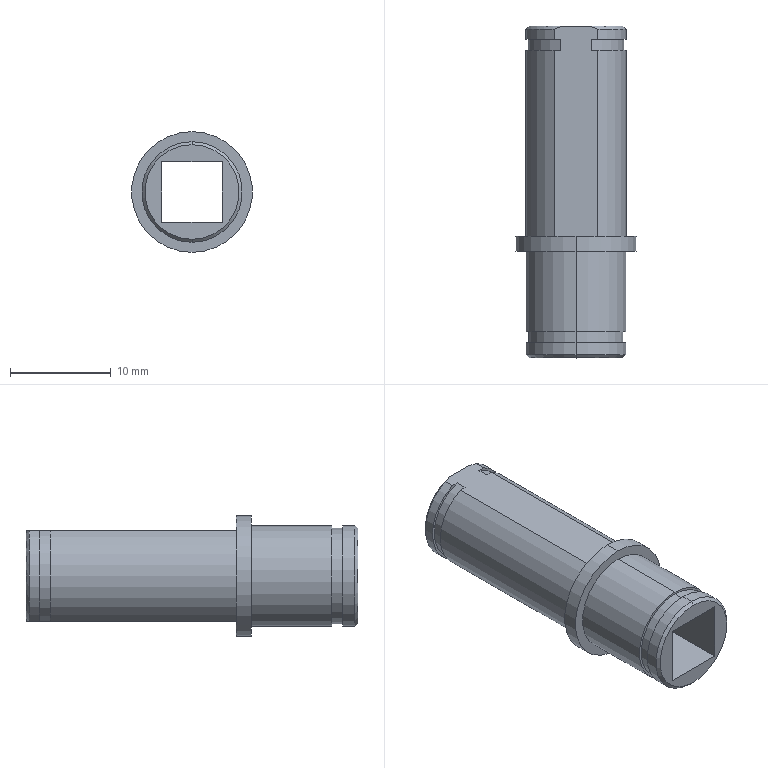Part | NX | features BREP 1 | 1 solid | 34 faces | box 12 x 33 x 12 mm | volume 1377 mm3 | plane 16 | cylinder 14 | cone 4 | commonest cylinder face diameters 10 x8 9.5 x4 12 x2
STEP:
#1=CARTESIAN_POINT('',(0.,0.3,-5.));
#2=VERTEX_POINT('',#1);
#3=CARTESIAN_POINT('',(0.,0.,-4.7));
#4=VERTEX_POINT('',#3);
#5=CARTESIAN_POINT('',(0.,0.,-4.7));
#6=DIRECTION('',(0.,0.7071,-0.7071));
#7=VECTOR('',#6,1000.);
#8=LINE('',#5,#7);
#9=EDGE_CURVE('',#2,#4,#8,.F.);
#10=ORIENTED_EDGE('',*,*,#9,.T.);
#11=CARTESIAN_POINT('',(0.,0.,4.7));
#12=VERTEX_POINT('',#11);
#13=CARTESIAN_POINT('',(0.,0.,0.));
#14=DIRECTION('',(0.,-1.,0.));
#15=DIRECTION('',(0.,0.,1.));
#16=AXIS2_PLACEMENT_3D('',#13,#14,#15);
#17=CIRCLE('',#16,4.7);
#18=EDGE_CURVE('',#12,#4,#17,.T.);
#19=ORIENTED_EDGE('',*,*,#18,.F.);
#20=CARTESIAN_POINT('',(0.,0.3,5.));
#21=VERTEX_POINT('',#20);
#22=CARTESIAN_POINT('',(0.,0.,4.7));
#23=DIRECTION('',(0.,0.7071,0.7071));
#24=VECTOR('',#23,1000.);
#25=LINE('',#22,#24);
#26=EDGE_CURVE('',#21,#12,#25,.F.);
#27=ORIENTED_EDGE('',*,*,#26,.F.);
#28=CARTESIAN_POINT('',(0.,0.3,0.));
#29=DIRECTION('',(0.,1.,0.));
#30=DIRECTION('',(0.,0.,1.));
#31=AXIS2_PLACEMENT_3D('',#28,#29,#30);
#32=CIRCLE('',#31,5.);
#33=EDGE_CURVE('',#2,#21,#32,.T.);
#34=ORIENTED_EDGE('',*,*,#33,.F.);
#35=EDGE_LOOP('',(#10,#19,#27,#34));
#36=FACE_BOUND('',#35,.T.);
#37=CARTESIAN_POINT('',(0.,0.,0.));
#38=DIRECTION('',(0.,1.,0.));
#39=DIRECTION('',(0.,0.,1.));
#40=AXIS2_PLACEMENT_3D('',#37,#38,#39);
#41=CONICAL_SURFACE('',#40,4.7,0.7854);
#42=ADVANCED_FACE('',(#36),#41,.T.);
#43=CARTESIAN_POINT('',(-1.356,33.,4.5));
#44=VERTEX_POINT('',#43);
#45=CARTESIAN_POINT('',(-2.179,32.7,4.5));
#46=VERTEX_POINT('',#45);
#47=CARTESIAN_POINT('',(-1.356,33.,4.5));
#48=CARTESIAN_POINT('',(-1.622,32.923,4.5));
#49=CARTESIAN_POINT('',(-1.897,32.823,4.5));
#50=CARTESIAN_POINT('',(-2.179,32.7,4.5));
#51=B_SPLINE_CURVE_WITH_KNOTS('',3,(#47,#48,#49,#50),.UNSPECIFIED.,.F.,.F.,(4,4),(0.,1.),.UNSPECIFIED.);
#52=EDGE_CURVE('',#44,#46,#51,.T.);
#53=ORIENTED_EDGE('',*,*,#52,.F.);
#54=CARTESIAN_POINT('',(-1.356,33.,-4.5));
#55=VERTEX_POINT('',#54);
#56=CARTESIAN_POINT('',(0.,33.,0.));
#57=DIRECTION('',(0.,1.,0.));
#58=DIRECTION('',(0.,0.,-1.));
#59=AXIS2_PLACEMENT_3D('',#56,#57,#58);
#60=CIRCLE('',#59,4.7);
#61=EDGE_CURVE('',#55,#44,#60,.T.);
#62=ORIENTED_EDGE('',*,*,#61,.F.);
#63=CARTESIAN_POINT('',(-2.179,32.7,-4.5));
#64=VERTEX_POINT('',#63);
#65=CARTESIAN_POINT('',(-2.179,32.7,-4.5));
#66=CARTESIAN_POINT('',(-1.897,32.823,-4.5));
#67=CARTESIAN_POINT('',(-1.622,32.923,-4.5));
#68=CARTESIAN_POINT('',(-1.356,33.,-4.5));
#69=B_SPLINE_CURVE_WITH_KNOTS('',3,(#65,#66,#67,#68),.UNSPECIFIED.,.F.,.F.,(4,4),(0.,1.),.UNSPECIFIED.);
#70=EDGE_CURVE('',#64,#55,#69,.T.);
#71=ORIENTED_EDGE('',*,*,#70,.F.);
#72=CARTESIAN_POINT('',(0.,32.7,0.));
#73=DIRECTION('',(0.,-1.,0.));
#74=DIRECTION('',(0.,0.,-1.));
#75=AXIS2_PLACEMENT_3D('',#72,#73,#74);
#76=CIRCLE('',#75,5.);
#77=EDGE_CURVE('',#46,#64,#76,.T.);
#78=ORIENTED_EDGE('',*,*,#77,.F.);
#79=EDGE_LOOP('',(#53,#62,#71,#78));
#80=FACE_BOUND('',#79,.T.);
#81=CARTESIAN_POINT('',(0.,32.7,0.));
#82=DIRECTION('',(0.,-1.,0.));
#83=DIRECTION('',(0.,0.,-1.));
#84=AXIS2_PLACEMENT_3D('',#81,#82,#83);
#85=CONICAL_SURFACE('',#84,5.,0.7854);
#86=ADVANCED_FACE('',(#80),#85,.T.);
#87=CARTESIAN_POINT('',(1.356,33.,-4.5));
#88=VERTEX_POINT('',#87);
#89=CARTESIAN_POINT('',(2.179,32.7,-4.5));
#90=VERTEX_POINT('',#89);
#91=CARTESIAN_POINT('',(1.356,33.,-4.5));
#92=CARTESIAN_POINT('',(1.622,32.923,-4.5));
#93=CARTESIAN_POINT('',(1.897,32.823,-4.5));
#94=CARTESIAN_POINT('',(2.179,32.7,-4.5));
#95=B_SPLINE_CURVE_WITH_KNOTS('',3,(#91,#92,#93,#94),.UNSPECIFIED.,.F.,.F.,(4,4),(0.,1.),.UNSPECIFIED.);
#96=EDGE_CURVE('',#88,#90,#95,.T.);
#97=ORIENTED_EDGE('',*,*,#96,.F.);
#98=CARTESIAN_POINT('',(1.356,33.,4.5));
#99=VERTEX_POINT('',#98);
#100=CARTESIAN_POINT('',(0.,33.,0.));
#101=DIRECTION('',(0.,1.,0.));
#102=DIRECTION('',(0.,0.,-1.));
#103=AXIS2_PLACEMENT_3D('',#100,#101,#102);
#104=CIRCLE('',#103,4.7);
#105=EDGE_CURVE('',#99,#88,#104,.T.);
#106=ORIENTED_EDGE('',*,*,#105,.F.);
#107=CARTESIAN_POINT('',(2.179,32.7,4.5));
#108=VERTEX_POINT('',#107);
#109=CARTESIAN_POINT('',(2.179,32.7,4.5));
#110=CARTESIAN_POINT('',(1.897,32.823,4.5));
#111=CARTESIAN_POINT('',(1.622,32.923,4.5));
#112=CARTESIAN_POINT('',(1.356,33.,4.5));
#113=B_SPLINE_CURVE_WITH_KNOTS('',3,(#109,#110,#111,#112),.UNSPECIFIED.,.F.,.F.,(4,4),(0.,1.),.UNSPECIFIED.);
#114=EDGE_CURVE('',#108,#99,#113,.T.);
#115=ORIENTED_EDGE('',*,*,#114,.F.);
#116=CARTESIAN_POINT('',(0.,32.7,0.));
#117=DIRECTION('',(0.,-1.,0.));
#118=DIRECTION('',(0.,0.,-1.));
#119=AXIS2_PLACEMENT_3D('',#116,#117,#118);
#120=CIRCLE('',#119,5.);
#121=EDGE_CURVE('',#90,#108,#120,.T.);
#122=ORIENTED_EDGE('',*,*,#121,.F.);
#123=EDGE_LOOP('',(#97,#106,#115,#122));
#124=FACE_BOUND('',#123,.T.);
#125=CARTESIAN_POINT('',(0.,32.7,0.));
#126=DIRECTION('',(0.,-1.,0.));
#127=DIRECTION('',(0.,0.,-1.));
#128=AXIS2_PLACEMENT_3D('',#125,#126,#127);
#129=CONICAL_SURFACE('',#128,5.,0.7854);
#130=ADVANCED_FACE('',(#124),#129,.T.);
#131=CARTESIAN_POINT('',(2.179,33.,-4.5));
#132=DIRECTION('',(1.,0.,0.));
#133=VECTOR('',#132,1000.);
#134=LINE('',#131,#133);
#135=EDGE_CURVE('',#55,#88,#134,.T.);
#136=ORIENTED_EDGE('',*,*,#135,.T.);
#137=ORIENTED_EDGE('',*,*,#96,.T.);
#138=CARTESIAN_POINT('',(2.179,31.7,-4.5));
#139=VERTEX_POINT('',#138);
#140=CARTESIAN_POINT('',(2.179,7.47,-4.5));
#141=DIRECTION('',(0.,1.,0.));
#142=VECTOR('',#141,1000.);
#143=LINE('',#140,#142);
#144=EDGE_CURVE('',#139,#90,#143,.T.);
#145=ORIENTED_EDGE('',*,*,#144,.F.);
#146=CARTESIAN_POINT('',(1.521,31.7,-4.5));
#147=VERTEX_POINT('',#146);
#148=CARTESIAN_POINT('',(0.,31.7,-4.5));
#149=DIRECTION('',(1.,0.,0.));
#150=VECTOR('',#149,1000.);
#151=LINE('',#148,#150);
#152=EDGE_CURVE('',#147,#139,#151,.T.);
#153=ORIENTED_EDGE('',*,*,#152,.F.);
#154=CARTESIAN_POINT('',(1.521,30.6,-4.5));
#155=VERTEX_POINT('',#154);
#156=CARTESIAN_POINT('',(1.521,31.7,-4.5));
#157=DIRECTION('',(0.,1.,0.));
#158=VECTOR('',#157,1000.);
#159=LINE('',#156,#158);
#160=EDGE_CURVE('',#155,#147,#159,.T.);
#161=ORIENTED_EDGE('',*,*,#160,.F.);
#162=CARTESIAN_POINT('',(2.179,30.6,-4.5));
#163=VERTEX_POINT('',#162);
#164=CARTESIAN_POINT('',(0.,30.6,-4.5));
#165=DIRECTION('',(1.,0.,0.));
#166=VECTOR('',#165,1000.);
#167=LINE('',#164,#166);
#168=EDGE_CURVE('',#155,#163,#167,.T.);
#169=ORIENTED_EDGE('',*,*,#168,.T.);
#170=CARTESIAN_POINT('',(2.179,12.1,-4.5));
#171=VERTEX_POINT('',#170);
#172=CARTESIAN_POINT('',(2.179,7.47,-4.5));
#173=DIRECTION('',(0.,1.,0.));
#174=VECTOR('',#173,1000.);
#175=LINE('',#172,#174);
#176=EDGE_CURVE('',#171,#163,#175,.T.);
#177=ORIENTED_EDGE('',*,*,#176,.F.);
#178=CARTESIAN_POINT('',(-2.179,12.1,-4.5));
#179=VERTEX_POINT('',#178);
#180=CARTESIAN_POINT('',(2.179,12.1,-4.5));
#181=DIRECTION('',(1.,0.,0.));
#182=VECTOR('',#181,1000.);
#183=LINE('',#180,#182);
#184=EDGE_CURVE('',#179,#171,#183,.T.);
#185=ORIENTED_EDGE('',*,*,#184,.F.);
#186=CARTESIAN_POINT('',(-2.179,30.6,-4.5));
#187=VERTEX_POINT('',#186);
#188=CARTESIAN_POINT('',(-2.179,7.47,-4.5));
#189=DIRECTION('',(0.,1.,0.));
#190=VECTOR('',#189,1000.);
#191=LINE('',#188,#190);
#192=EDGE_CURVE('',#179,#187,#191,.T.);
#193=ORIENTED_EDGE('',*,*,#192,.T.);
#194=CARTESIAN_POINT('',(-1.521,30.6,-4.5));
#195=VERTEX_POINT('',#194);
#196=CARTESIAN_POINT('',(0.,30.6,-4.5));
#197=DIRECTION('',(1.,0.,0.));
#198=VECTOR('',#197,1000.);
#199=LINE('',#196,#198);
#200=EDGE_CURVE('',#187,#195,#199,.T.);
#201=ORIENTED_EDGE('',*,*,#200,.T.);
#202=CARTESIAN_POINT('',(-1.521,31.7,-4.5));
#203=VERTEX_POINT('',#202);
#204=CARTESIAN_POINT('',(-1.521,31.7,-4.5));
#205=DIRECTION('',(0.,-1.,0.));
#206=VECTOR('',#205,1000.);
#207=LINE('',#204,#206);
#208=EDGE_CURVE('',#203,#195,#207,.T.);
#209=ORIENTED_EDGE('',*,*,#208,.F.);
#210=CARTESIAN_POINT('',(-2.179,31.7,-4.5));
#211=VERTEX_POINT('',#210);
#212=CARTESIAN_POINT('',(0.,31.7,-4.5));
#213=DIRECTION('',(1.,0.,0.));
#214=VECTOR('',#213,1000.);
#215=LINE('',#212,#214);
#216=EDGE_CURVE('',#211,#203,#215,.T.);
#217=ORIENTED_EDGE('',*,*,#216,.F.);
#218=CARTESIAN_POINT('',(-2.179,7.47,-4.5));
#219=DIRECTION('',(0.,1.,0.));
#220=VECTOR('',#219,1000.);
#221=LINE('',#218,#220);
#222=EDGE_CURVE('',#211,#64,#221,.T.);
#223=ORIENTED_EDGE('',*,*,#222,.T.);
#224=ORIENTED_EDGE('',*,*,#70,.T.);
#225=EDGE_LOOP('',(#136,#137,#145,#153,#161,#169,#177,#185,#193,#201,#209,#217,#223,#224));
#226=FACE_BOUND('',#225,.T.);
#227=CARTESIAN_POINT('',(2.179,7.47,-4.5));
#228=DIRECTION('',(0.,0.,1.));
#229=DIRECTION('',(1.,0.,0.));
#230=AXIS2_PLACEMENT_3D('',#227,#228,#229);
#231=PLANE('',#230);
#232=ADVANCED_FACE('',(#226),#231,.F.);
#233=CARTESIAN_POINT('',(2.179,31.7,4.5));
#234=VERTEX_POINT('',#233);
#235=CARTESIAN_POINT('',(2.179,7.47,4.5));
#236=DIRECTION('',(0.,1.,0.));
#237=VECTOR('',#236,1000.);
#238=LINE('',#235,#237);
#239=EDGE_CURVE('',#234,#108,#238,.T.);
#240=ORIENTED_EDGE('',*,*,#239,.T.);
#241=ORIENTED_EDGE('',*,*,#114,.T.);
#242=CARTESIAN_POINT('',(2.179,33.,4.5));
#243=DIRECTION('',(-1.,0.,0.));
#244=VECTOR('',#243,1000.);
#245=LINE('',#242,#244);
#246=EDGE_CURVE('',#99,#44,#245,.T.);
#247=ORIENTED_EDGE('',*,*,#246,.T.);
#248=ORIENTED_EDGE('',*,*,#52,.T.);
#249=CARTESIAN_POINT('',(-2.179,31.7,4.5));
#250=VERTEX_POINT('',#249);
#251=CARTESIAN_POINT('',(-2.179,7.47,4.5));
#252=DIRECTION('',(0.,1.,0.));
#253=VECTOR('',#252,1000.);
#254=LINE('',#251,#253);
#255=EDGE_CURVE('',#250,#46,#254,.T.);
#256=ORIENTED_EDGE('',*,*,#255,.F.);
#257=CARTESIAN_POINT('',(-1.521,31.7,4.5));
#258=VERTEX_POINT('',#257);
#259=CARTESIAN_POINT('',(0.,31.7,4.5));
#260=DIRECTION('',(-1.,0.,0.));
#261=VECTOR('',#260,1000.);
#262=LINE('',#259,#261);
#263=EDGE_CURVE('',#258,#250,#262,.T.);
#264=ORIENTED_EDGE('',*,*,#263,.F.);
#265=CARTESIAN_POINT('',(-1.521,30.6,4.5));
#266=VERTEX_POINT('',#265);
#267=CARTESIAN_POINT('',(-1.521,31.7,4.5));
#268=DIRECTION('',(0.,1.,0.));
#269=VECTOR('',#268,1000.);
#270=LINE('',#267,#269);
#271=EDGE_CURVE('',#266,#258,#270,.T.);
#272=ORIENTED_EDGE('',*,*,#271,.F.);
#273=CARTESIAN_POINT('',(-2.179,30.6,4.5));
#274=VERTEX_POINT('',#273);
#275=CARTESIAN_POINT('',(0.,30.6,4.5));
#276=DIRECTION('',(-1.,0.,0.));
#277=VECTOR('',#276,1000.);
#278=LINE('',#275,#277);
#279=EDGE_CURVE('',#266,#274,#278,.T.);
#280=ORIENTED_EDGE('',*,*,#279,.T.);
#281=CARTESIAN_POINT('',(-2.179,12.1,4.5));
#282=VERTEX_POINT('',#281);
#283=CARTESIAN_POINT('',(-2.179,7.47,4.5));
#284=DIRECTION('',(0.,1.,0.));
#285=VECTOR('',#284,1000.);
#286=LINE('',#283,#285);
#287=EDGE_CURVE('',#282,#274,#286,.T.);
#288=ORIENTED_EDGE('',*,*,#287,.F.);
#289=CARTESIAN_POINT('',(2.179,12.1,4.5));
#290=VERTEX_POINT('',#289);
#291=CARTESIAN_POINT('',(2.179,12.1,4.5));
#292=DIRECTION('',(-1.,0.,0.));
#293=VECTOR('',#292,1000.);
#294=LINE('',#291,#293);
#295=EDGE_CURVE('',#290,#282,#294,.T.);
#296=ORIENTED_EDGE('',*,*,#295,.F.);
#297=CARTESIAN_POINT('',(2.179,30.6,4.5));
#298=VERTEX_POINT('',#297);
#299=CARTESIAN_POINT('',(2.179,7.47,4.5));
#300=DIRECTION('',(0.,1.,0.));
#301=VECTOR('',#300,1000.);
#302=LINE('',#299,#301);
#303=EDGE_CURVE('',#290,#298,#302,.T.);
#304=ORIENTED_EDGE('',*,*,#303,.T.);
#305=CARTESIAN_POINT('',(1.521,30.6,4.5));
#306=VERTEX_POINT('',#305);
#307=CARTESIAN_POINT('',(0.,30.6,4.5));
#308=DIRECTION('',(-1.,0.,0.));
#309=VECTOR('',#308,1000.);
#310=LINE('',#307,#309);
#311=EDGE_CURVE('',#298,#306,#310,.T.);
#312=ORIENTED_EDGE('',*,*,#311,.T.);
#313=CARTESIAN_POINT('',(1.521,31.7,4.5));
#314=VERTEX_POINT('',#313);
#315=CARTESIAN_POINT('',(1.521,31.7,4.5));
#316=DIRECTION('',(0.,-1.,0.));
#317=VECTOR('',#316,1000.);
#318=LINE('',#315,#317);
#319=EDGE_CURVE('',#314,#306,#318,.T.);
#320=ORIENTED_EDGE('',*,*,#319,.F.);
#321=CARTESIAN_POINT('',(0.,31.7,4.5));
#322=DIRECTION('',(-1.,0.,0.));
#323=VECTOR('',#322,1000.);
#324=LINE('',#321,#323);
#325=EDGE_CURVE('',#234,#314,#324,.T.);
#326=ORIENTED_EDGE('',*,*,#325,.F.);
#327=EDGE_LOOP('',(#240,#241,#247,#248,#256,#264,#272,#280,#288,#296,#304,#312,#320,#326));
#328=FACE_BOUND('',#327,.T.);
#329=CARTESIAN_POINT('',(2.179,7.47,4.5));
#330=DIRECTION('',(0.,0.,-1.));
#331=DIRECTION('',(-1.,0.,0.));
#332=AXIS2_PLACEMENT_3D('',#329,#330,#331);
#333=PLANE('',#332);
#334=ADVANCED_FACE('',(#328),#333,.F.);
#335=CARTESIAN_POINT('',(0.,30.6,0.));
#336=DIRECTION('',(0.,1.,0.));
#337=DIRECTION('',(0.,0.,1.));
#338=AXIS2_PLACEMENT_3D('',#335,#336,#337);
#339=CIRCLE('',#338,4.75);
#340=EDGE_CURVE('',#306,#155,#339,.T.);
#341=ORIENTED_EDGE('',*,*,#340,.T.);
#342=ORIENTED_EDGE('',*,*,#160,.T.);
#343=CARTESIAN_POINT('',(0.,31.7,0.));
#344=DIRECTION('',(0.,1.,0.));
#345=DIRECTION('',(0.,0.,1.));
#346=AXIS2_PLACEMENT_3D('',#343,#344,#345);
#347=CIRCLE('',#346,4.75);
#348=EDGE_CURVE('',#314,#147,#347,.T.);
#349=ORIENTED_EDGE('',*,*,#348,.F.);
#350=ORIENTED_EDGE('',*,*,#319,.T.);
#351=EDGE_LOOP('',(#341,#342,#349,#350));
#352=FACE_BOUND('',#351,.T.);
#353=CARTESIAN_POINT('',(0.,31.7,0.));
#354=DIRECTION('',(0.,-1.,0.));
#355=DIRECTION('',(0.,0.,-1.));
#356=AXIS2_PLACEMENT_3D('',#353,#354,#355);
#357=CYLINDRICAL_SURFACE('',#356,4.75);
#358=ADVANCED_FACE('',(#352),#357,.T.);
#359=ORIENTED_EDGE('',*,*,#168,.F.);
#360=ORIENTED_EDGE('',*,*,#340,.F.);
#361=ORIENTED_EDGE('',*,*,#311,.F.);
#362=CARTESIAN_POINT('',(0.,30.6,0.));
#363=DIRECTION('',(0.,1.,0.));
#364=DIRECTION('',(0.,0.,1.));
#365=AXIS2_PLACEMENT_3D('',#362,#363,#364);
#366=CIRCLE('',#365,5.);
#367=EDGE_CURVE('',#298,#163,#366,.T.);
#368=ORIENTED_EDGE('',*,*,#367,.T.);
#369=EDGE_LOOP('',(#359,#360,#361,#368));
#370=FACE_BOUND('',#369,.T.);
#371=CARTESIAN_POINT('',(0.,30.6,0.));
#372=DIRECTION('',(0.,1.,0.));
#373=DIRECTION('',(0.,0.,1.));
#374=AXIS2_PLACEMENT_3D('',#371,#372,#373);
#375=PLANE('',#374);
#376=ADVANCED_FACE('',(#370),#375,.T.);
#377=ORIENTED_EDGE('',*,*,#348,.T.);
#378=ORIENTED_EDGE('',*,*,#152,.T.);
#379=CARTESIAN_POINT('',(0.,31.7,0.));
#380=DIRECTION('',(0.,1.,0.));
#381=DIRECTION('',(0.,0.,1.));
#382=AXIS2_PLACEMENT_3D('',#379,#380,#381);
#383=CIRCLE('',#382,5.);
#384=EDGE_CURVE('',#234,#139,#383,.T.);
#385=ORIENTED_EDGE('',*,*,#384,.F.);
#386=ORIENTED_EDGE('',*,*,#325,.T.);
#387=EDGE_LOOP('',(#377,#378,#385,#386));
#388=FACE_BOUND('',#387,.T.);
#389=CARTESIAN_POINT('',(0.,31.7,0.));
#390=DIRECTION('',(0.,1.,0.));
#391=DIRECTION('',(0.,0.,1.));
#392=AXIS2_PLACEMENT_3D('',#389,#390,#391);
#393=PLANE('',#392);
#394=ADVANCED_FACE('',(#388),#393,.F.);
#395=CARTESIAN_POINT('',(3.,33.,3.));
#396=VERTEX_POINT('',#395);
#397=CARTESIAN_POINT('',(3.,0.,3.));
#398=VERTEX_POINT('',#397);
#399=CARTESIAN_POINT('',(3.,40.,3.));
#400=DIRECTION('',(0.,-1.,0.));
#401=VECTOR('',#400,1000.);
#402=LINE('',#399,#401);
#403=EDGE_CURVE('',#396,#398,#402,.T.);
#404=ORIENTED_EDGE('',*,*,#403,.T.);
#405=CARTESIAN_POINT('',(-3.,0.,3.));
#406=VERTEX_POINT('',#405);
#407=CARTESIAN_POINT('',(-3.,0.,3.));
#408=DIRECTION('',(-1.,0.,0.));
#409=VECTOR('',#408,1000.);
#410=LINE('',#407,#409);
#411=EDGE_CURVE('',#398,#406,#410,.T.);
#412=ORIENTED_EDGE('',*,*,#411,.T.);
#413=CARTESIAN_POINT('',(-3.,33.,3.));
#414=VERTEX_POINT('',#413);
#415=CARTESIAN_POINT('',(-3.,40.,3.));
#416=DIRECTION('',(0.,-1.,0.));
#417=VECTOR('',#416,1000.);
#418=LINE('',#415,#417);
#419=EDGE_CURVE('',#414,#406,#418,.T.);
#420=ORIENTED_EDGE('',*,*,#419,.F.);
#421=CARTESIAN_POINT('',(-5.,33.,3.));
#422=DIRECTION('',(-1.,0.,0.));
#423=VECTOR('',#422,1000.);
#424=LINE('',#421,#423);
#425=EDGE_CURVE('',#396,#414,#424,.T.);
#426=ORIENTED_EDGE('',*,*,#425,.F.);
#427=EDGE_LOOP('',(#404,#412,#420,#426));
#428=FACE_BOUND('',#427,.T.);
#429=CARTESIAN_POINT('',(-3.,40.,3.));
#430=DIRECTION('',(0.,0.,1.));
#431=DIRECTION('',(1.,0.,0.));
#432=AXIS2_PLACEMENT_3D('',#429,#430,#431);
#433=PLANE('',#432);
#434=ADVANCED_FACE('',(#428),#433,.F.);
#435=ORIENTED_EDGE('',*,*,#419,.T.);
#436=CARTESIAN_POINT('',(-3.,0.,-3.));
#437=VERTEX_POINT('',#436);
#438=CARTESIAN_POINT('',(-3.,0.,-3.));
#439=DIRECTION('',(0.,0.,-1.));
#440=VECTOR('',#439,1000.);
#441=LINE('',#438,#440);
#442=EDGE_CURVE('',#406,#437,#441,.T.);
#443=ORIENTED_EDGE('',*,*,#442,.T.);
#444=CARTESIAN_POINT('',(-3.,33.,-3.));
#445=VERTEX_POINT('',#444);
#446=CARTESIAN_POINT('',(-3.,40.,-3.));
#447=DIRECTION('',(0.,-1.,0.));
#448=VECTOR('',#447,1000.);
#449=LINE('',#446,#448);
#450=EDGE_CURVE('',#445,#437,#449,.T.);
#451=ORIENTED_EDGE('',*,*,#450,.F.);
#452=CARTESIAN_POINT('',(-3.,33.,0.));
#453=DIRECTION('',(0.,0.,-1.));
#454=VECTOR('',#453,1000.);
#455=LINE('',#452,#454);
#456=EDGE_CURVE('',#414,#445,#455,.T.);
#457=ORIENTED_EDGE('',*,*,#456,.F.);
#458=EDGE_LOOP('',(#435,#443,#451,#457));
#459=FACE_BOUND('',#458,.T.);
#460=CARTESIAN_POINT('',(-3.,40.,-3.));
#461=DIRECTION('',(-1.,0.,0.));
#462=DIRECTION('',(0.,0.,1.));
#463=AXIS2_PLACEMENT_3D('',#460,#461,#462);
#464=PLANE('',#463);
#465=ADVANCED_FACE('',(#459),#464,.F.);
#466=ORIENTED_EDGE('',*,*,#450,.T.);
#467=CARTESIAN_POINT('',(3.,0.,-3.));
#468=VERTEX_POINT('',#467);
#469=CARTESIAN_POINT('',(-3.,0.,-3.));
#470=DIRECTION('',(1.,0.,0.));
#471=VECTOR('',#470,1000.);
#472=LINE('',#469,#471);
#473=EDGE_CURVE('',#437,#468,#472,.T.);
#474=ORIENTED_EDGE('',*,*,#473,.T.);
#475=CARTESIAN_POINT('',(3.,33.,-3.));
#476=VERTEX_POINT('',#475);
#477=CARTESIAN_POINT('',(3.,40.,-3.));
#478=DIRECTION('',(0.,-1.,0.));
#479=VECTOR('',#478,1000.);
#480=LINE('',#477,#479);
#481=EDGE_CURVE('',#476,#468,#480,.T.);
#482=ORIENTED_EDGE('',*,*,#481,.F.);
#483=CARTESIAN_POINT('',(-5.,33.,-3.));
#484=DIRECTION('',(1.,0.,0.));
#485=VECTOR('',#484,1000.);
#486=LINE('',#483,#485);
#487=EDGE_CURVE('',#445,#476,#486,.T.);
#488=ORIENTED_EDGE('',*,*,#487,.F.);
#489=EDGE_LOOP('',(#466,#474,#482,#488));
#490=FACE_BOUND('',#489,.T.);
#491=CARTESIAN_POINT('',(-3.,40.,-3.));
#492=DIRECTION('',(0.,0.,-1.));
#493=DIRECTION('',(-1.,0.,0.));
#494=AXIS2_PLACEMENT_3D('',#491,#492,#493);
#495=PLANE('',#494);
#496=ADVANCED_FACE('',(#490),#495,.F.);
#497=ORIENTED_EDGE('',*,*,#481,.T.);
#498=CARTESIAN_POINT('',(3.,0.,-3.));
#499=DIRECTION('',(0.,0.,1.));
#500=VECTOR('',#499,1000.);
#501=LINE('',#498,#500);
#502=EDGE_CURVE('',#468,#398,#501,.T.);
#503=ORIENTED_EDGE('',*,*,#502,.T.);
#504=ORIENTED_EDGE('',*,*,#403,.F.);
#505=CARTESIAN_POINT('',(3.,33.,0.));
#506=DIRECTION('',(0.,0.,1.));
#507=VECTOR('',#506,1000.);
#508=LINE('',#505,#507);
#509=EDGE_CURVE('',#476,#396,#508,.T.);
#510=ORIENTED_EDGE('',*,*,#509,.F.);
#511=EDGE_LOOP('',(#497,#503,#504,#510));
#512=FACE_BOUND('',#511,.T.);
#513=CARTESIAN_POINT('',(3.,40.,-3.));
#514=DIRECTION('',(1.,0.,0.));
#515=DIRECTION('',(0.,0.,-1.));
#516=AXIS2_PLACEMENT_3D('',#513,#514,#515);
#517=PLANE('',#516);
#518=ADVANCED_FACE('',(#512),#517,.F.);
#519=ORIENTED_EDGE('',*,*,#246,.F.);
#520=ORIENTED_EDGE('',*,*,#105,.T.);
#521=ORIENTED_EDGE('',*,*,#135,.F.);
#522=ORIENTED_EDGE('',*,*,#61,.T.);
#523=EDGE_LOOP('',(#519,#520,#521,#522));
#524=FACE_BOUND('',#523,.T.);
#525=ORIENTED_EDGE('',*,*,#487,.T.);
#526=ORIENTED_EDGE('',*,*,#509,.T.);
#527=ORIENTED_EDGE('',*,*,#425,.T.);
#528=ORIENTED_EDGE('',*,*,#456,.T.);
#529=EDGE_LOOP('',(#525,#526,#527,#528));
#530=FACE_BOUND('',#529,.T.);
#531=CARTESIAN_POINT('',(-5.,33.,0.));
#532=DIRECTION('',(0.,-1.,0.));
#533=DIRECTION('',(0.,0.,-1.));
#534=AXIS2_PLACEMENT_3D('',#531,#532,#533);
#535=PLANE('',#534);
#536=ADVANCED_FACE('',(#524,#530),#535,.F.);
#537=ORIENTED_EDGE('',*,*,#144,.T.);
#538=ORIENTED_EDGE('',*,*,#121,.T.);
#539=ORIENTED_EDGE('',*,*,#239,.F.);
#540=ORIENTED_EDGE('',*,*,#384,.T.);
#541=EDGE_LOOP('',(#537,#538,#539,#540));
#542=FACE_BOUND('',#541,.T.);
#543=CARTESIAN_POINT('',(0.,0.,0.));
#544=DIRECTION('',(0.,-1.,0.));
#545=DIRECTION('',(0.,0.,-1.));
#546=AXIS2_PLACEMENT_3D('',#543,#544,#545);
#547=CYLINDRICAL_SURFACE('',#546,5.);
#548=ADVANCED_FACE('',(#542),#547,.T.);
#549=CARTESIAN_POINT('',(0.,12.1,-6.));
#550=VERTEX_POINT('',#549);
#551=CARTESIAN_POINT('',(0.,12.1,6.));
#552=VERTEX_POINT('',#551);
#553=CARTESIAN_POINT('',(0.,12.1,0.));
#554=DIRECTION('',(0.,-1.,0.));
#555=DIRECTION('',(0.,0.,-1.));
#556=AXIS2_PLACEMENT_3D('',#553,#554,#555);
#557=CIRCLE('',#556,6.);
#558=EDGE_CURVE('',#550,#552,#557,.T.);
#559=ORIENTED_EDGE('',*,*,#558,.F.);
#560=CARTESIAN_POINT('',(0.,12.1,0.));
#561=DIRECTION('',(0.,-1.,0.));
#562=DIRECTION('',(0.,0.,-1.));
#563=AXIS2_PLACEMENT_3D('',#560,#561,#562);
#564=CIRCLE('',#563,6.);
#565=EDGE_CURVE('',#552,#550,#564,.T.);
#566=ORIENTED_EDGE('',*,*,#565,.F.);
#567=EDGE_LOOP('',(#559,#566));
#568=FACE_BOUND('',#567,.T.);
#569=CARTESIAN_POINT('',(0.,12.1,0.));
#570=DIRECTION('',(0.,-1.,0.));
#571=DIRECTION('',(0.,0.,-1.));
#572=AXIS2_PLACEMENT_3D('',#569,#570,#571);
#573=CIRCLE('',#572,5.);
#574=EDGE_CURVE('',#282,#179,#573,.T.);
#575=ORIENTED_EDGE('',*,*,#574,.T.);
#576=ORIENTED_EDGE('',*,*,#184,.T.);
#577=CARTESIAN_POINT('',(0.,12.1,0.));
#578=DIRECTION('',(0.,-1.,0.));
#579=DIRECTION('',(0.,0.,-1.));
#580=AXIS2_PLACEMENT_3D('',#577,#578,#579);
#581=CIRCLE('',#580,5.);
#582=EDGE_CURVE('',#171,#290,#581,.T.);
#583=ORIENTED_EDGE('',*,*,#582,.T.);
#584=ORIENTED_EDGE('',*,*,#295,.T.);
#585=EDGE_LOOP('',(#575,#576,#583,#584));
#586=FACE_BOUND('',#585,.T.);
#587=CARTESIAN_POINT('',(-6.,12.1,0.));
#588=DIRECTION('',(0.,-1.,0.));
#589=DIRECTION('',(0.,0.,-1.));
#590=AXIS2_PLACEMENT_3D('',#587,#588,#589);
#591=PLANE('',#590);
#592=ADVANCED_FACE('',(#568,#586),#591,.F.);
#593=CARTESIAN_POINT('',(0.,10.6,6.));
#594=VERTEX_POINT('',#593);
#595=CARTESIAN_POINT('',(0.,0.,6.));
#596=DIRECTION('',(0.,-1.,0.));
#597=VECTOR('',#596,1000.);
#598=LINE('',#595,#597);
#599=EDGE_CURVE('',#552,#594,#598,.T.);
#600=ORIENTED_EDGE('',*,*,#599,.F.);
#601=ORIENTED_EDGE('',*,*,#565,.T.);
#602=CARTESIAN_POINT('',(0.,10.6,-6.));
#603=VERTEX_POINT('',#602);
#604=CARTESIAN_POINT('',(0.,0.,-6.));
#605=DIRECTION('',(0.,-1.,0.));
#606=VECTOR('',#605,1000.);
#607=LINE('',#604,#606);
#608=EDGE_CURVE('',#550,#603,#607,.T.);
#609=ORIENTED_EDGE('',*,*,#608,.T.);
#610=CARTESIAN_POINT('',(0.,10.6,0.));
#611=DIRECTION('',(0.,-1.,0.));
#612=DIRECTION('',(0.,0.,-1.));
#613=AXIS2_PLACEMENT_3D('',#610,#611,#612);
#614=CIRCLE('',#613,6.);
#615=EDGE_CURVE('',#594,#603,#614,.T.);
#616=ORIENTED_EDGE('',*,*,#615,.F.);
#617=EDGE_LOOP('',(#600,#601,#609,#616));
#618=FACE_BOUND('',#617,.T.);
#619=CARTESIAN_POINT('',(0.,0.,0.));
#620=DIRECTION('',(0.,-1.,0.));
#621=DIRECTION('',(0.,0.,-1.));
#622=AXIS2_PLACEMENT_3D('',#619,#620,#621);
#623=CYLINDRICAL_SURFACE('',#622,6.);
#624=ADVANCED_FACE('',(#618),#623,.T.);
#625=CARTESIAN_POINT('',(0.,10.6,0.));
#626=DIRECTION('',(0.,-1.,0.));
#627=DIRECTION('',(0.,0.,-1.));
#628=AXIS2_PLACEMENT_3D('',#625,#626,#627);
#629=CIRCLE('',#628,6.);
#630=EDGE_CURVE('',#603,#594,#629,.T.);
#631=ORIENTED_EDGE('',*,*,#630,.T.);
#632=ORIENTED_EDGE('',*,*,#615,.T.);
#633=EDGE_LOOP('',(#631,#632));
#634=FACE_BOUND('',#633,.T.);
#635=CARTESIAN_POINT('',(0.,10.6,-5.));
#636=VERTEX_POINT('',#635);
#637=CARTESIAN_POINT('',(0.,10.6,5.));
#638=VERTEX_POINT('',#637);
#639=CARTESIAN_POINT('',(0.,10.6,0.));
#640=DIRECTION('',(0.,-1.,0.));
#641=DIRECTION('',(0.,0.,-1.));
#642=AXIS2_PLACEMENT_3D('',#639,#640,#641);
#643=CIRCLE('',#642,5.);
#644=EDGE_CURVE('',#636,#638,#643,.T.);
#645=ORIENTED_EDGE('',*,*,#644,.F.);
#646=CARTESIAN_POINT('',(0.,10.6,0.));
#647=DIRECTION('',(0.,-1.,0.));
#648=DIRECTION('',(0.,0.,-1.));
#649=AXIS2_PLACEMENT_3D('',#646,#647,#648);
#650=CIRCLE('',#649,5.);
#651=EDGE_CURVE('',#638,#636,#650,.T.);
#652=ORIENTED_EDGE('',*,*,#651,.F.);
#653=EDGE_LOOP('',(#645,#652));
#654=FACE_BOUND('',#653,.T.);
#655=CARTESIAN_POINT('',(-5.,10.6,0.));
#656=DIRECTION('',(0.,1.,0.));
#657=DIRECTION('',(0.,0.,1.));
#658=AXIS2_PLACEMENT_3D('',#655,#656,#657);
#659=PLANE('',#658);
#660=ADVANCED_FACE('',(#634,#654),#659,.F.);
#661=CARTESIAN_POINT('',(0.,2.6,5.));
#662=VERTEX_POINT('',#661);
#663=CARTESIAN_POINT('',(0.,0.,5.));
#664=DIRECTION('',(0.,-1.,0.));
#665=VECTOR('',#664,1000.);
#666=LINE('',#663,#665);
#667=EDGE_CURVE('',#638,#662,#666,.T.);
#668=ORIENTED_EDGE('',*,*,#667,.F.);
#669=ORIENTED_EDGE('',*,*,#651,.T.);
#670=CARTESIAN_POINT('',(0.,2.6,-5.));
#671=VERTEX_POINT('',#670);
#672=CARTESIAN_POINT('',(0.,0.,-5.));
#673=DIRECTION('',(0.,-1.,0.));
#674=VECTOR('',#673,1000.);
#675=LINE('',#672,#674);
#676=EDGE_CURVE('',#636,#671,#675,.T.);
#677=ORIENTED_EDGE('',*,*,#676,.T.);
#678=CARTESIAN_POINT('',(0.,2.6,0.));
#679=DIRECTION('',(0.,-1.,0.));
#680=DIRECTION('',(0.,0.,-1.));
#681=AXIS2_PLACEMENT_3D('',#678,#679,#680);
#682=CIRCLE('',#681,5.);
#683=EDGE_CURVE('',#662,#671,#682,.T.);
#684=ORIENTED_EDGE('',*,*,#683,.F.);
#685=EDGE_LOOP('',(#668,#669,#677,#684));
#686=FACE_BOUND('',#685,.T.);
#687=CARTESIAN_POINT('',(0.,0.,0.));
#688=DIRECTION('',(0.,-1.,0.));
#689=DIRECTION('',(0.,0.,-1.));
#690=AXIS2_PLACEMENT_3D('',#687,#688,#689);
#691=CYLINDRICAL_SURFACE('',#690,5.);
#692=ADVANCED_FACE('',(#686),#691,.T.);
#693=CARTESIAN_POINT('',(0.,2.6,0.));
#694=DIRECTION('',(0.,-1.,0.));
#695=DIRECTION('',(0.,0.,-1.));
#696=AXIS2_PLACEMENT_3D('',#693,#694,#695);
#697=CIRCLE('',#696,5.);
#698=EDGE_CURVE('',#671,#662,#697,.T.);
#699=ORIENTED_EDGE('',*,*,#698,.T.);
#700=ORIENTED_EDGE('',*,*,#683,.T.);
#701=EDGE_LOOP('',(#699,#700));
#702=FACE_BOUND('',#701,.T.);
#703=CARTESIAN_POINT('',(0.,2.6,-4.75));
#704=VERTEX_POINT('',#703);
#705=CARTESIAN_POINT('',(0.,2.6,4.75));
#706=VERTEX_POINT('',#705);
#707=CARTESIAN_POINT('',(0.,2.6,0.));
#708=DIRECTION('',(0.,-1.,0.));
#709=DIRECTION('',(0.,0.,-1.));
#710=AXIS2_PLACEMENT_3D('',#707,#708,#709);
#711=CIRCLE('',#710,4.75);
#712=EDGE_CURVE('',#704,#706,#711,.T.);
#713=ORIENTED_EDGE('',*,*,#712,.F.);
#714=CARTESIAN_POINT('',(0.,2.6,0.));
#715=DIRECTION('',(0.,-1.,0.));
#716=DIRECTION('',(0.,0.,-1.));
#717=AXIS2_PLACEMENT_3D('',#714,#715,#716);
#718=CIRCLE('',#717,4.75);
#719=EDGE_CURVE('',#706,#704,#718,.T.);
#720=ORIENTED_EDGE('',*,*,#719,.F.);
#721=EDGE_LOOP('',(#713,#720));
#722=FACE_BOUND('',#721,.T.);
#723=CARTESIAN_POINT('',(-4.75,2.6,0.));
#724=DIRECTION('',(0.,1.,0.));
#725=DIRECTION('',(0.,0.,1.));
#726=AXIS2_PLACEMENT_3D('',#723,#724,#725);
#727=PLANE('',#726);
#728=ADVANCED_FACE('',(#702,#722),#727,.F.);
#729=CARTESIAN_POINT('',(0.,1.5,4.75));
#730=VERTEX_POINT('',#729);
#731=CARTESIAN_POINT('',(0.,0.,4.75));
#732=DIRECTION('',(0.,-1.,0.));
#733=VECTOR('',#732,1000.);
#734=LINE('',#731,#733);
#735=EDGE_CURVE('',#706,#730,#734,.T.);
#736=ORIENTED_EDGE('',*,*,#735,.F.);
#737=ORIENTED_EDGE('',*,*,#719,.T.);
#738=CARTESIAN_POINT('',(0.,1.5,-4.75));
#739=VERTEX_POINT('',#738);
#740=CARTESIAN_POINT('',(0.,0.,-4.75));
#741=DIRECTION('',(0.,-1.,0.));
#742=VECTOR('',#741,1000.);
#743=LINE('',#740,#742);
#744=EDGE_CURVE('',#704,#739,#743,.T.);
#745=ORIENTED_EDGE('',*,*,#744,.T.);
#746=CARTESIAN_POINT('',(0.,1.5,0.));
#747=DIRECTION('',(0.,-1.,0.));
#748=DIRECTION('',(0.,0.,-1.));
#749=AXIS2_PLACEMENT_3D('',#746,#747,#748);
#750=CIRCLE('',#749,4.75);
#751=EDGE_CURVE('',#730,#739,#750,.T.);
#752=ORIENTED_EDGE('',*,*,#751,.F.);
#753=EDGE_LOOP('',(#736,#737,#745,#752));
#754=FACE_BOUND('',#753,.T.);
#755=CARTESIAN_POINT('',(0.,0.,0.));
#756=DIRECTION('',(0.,-1.,0.));
#757=DIRECTION('',(0.,0.,-1.));
#758=AXIS2_PLACEMENT_3D('',#755,#756,#757);
#759=CYLINDRICAL_SURFACE('',#758,4.75);
#760=ADVANCED_FACE('',(#754),#759,.T.);
#761=CARTESIAN_POINT('',(0.,1.5,0.));
#762=DIRECTION('',(0.,-1.,0.));
#763=DIRECTION('',(0.,0.,-1.));
#764=AXIS2_PLACEMENT_3D('',#761,#762,#763);
#765=CIRCLE('',#764,4.75);
#766=EDGE_CURVE('',#739,#730,#765,.T.);
#767=ORIENTED_EDGE('',*,*,#766,.T.);
#768=ORIENTED_EDGE('',*,*,#751,.T.);
#769=EDGE_LOOP('',(#767,#768));
#770=FACE_BOUND('',#769,.T.);
#771=CARTESIAN_POINT('',(0.,1.5,-5.));
#772=VERTEX_POINT('',#771);
#773=CARTESIAN_POINT('',(0.,1.5,5.));
#774=VERTEX_POINT('',#773);
#775=CARTESIAN_POINT('',(0.,1.5,0.));
#776=DIRECTION('',(0.,-1.,0.));
#777=DIRECTION('',(0.,0.,-1.));
#778=AXIS2_PLACEMENT_3D('',#775,#776,#777);
#779=CIRCLE('',#778,5.);
#780=EDGE_CURVE('',#772,#774,#779,.T.);
#781=ORIENTED_EDGE('',*,*,#780,.F.);
#782=CARTESIAN_POINT('',(0.,1.5,0.));
#783=DIRECTION('',(0.,-1.,0.));
#784=DIRECTION('',(0.,0.,-1.));
#785=AXIS2_PLACEMENT_3D('',#782,#783,#784);
#786=CIRCLE('',#785,5.);
#787=EDGE_CURVE('',#774,#772,#786,.T.);
#788=ORIENTED_EDGE('',*,*,#787,.F.);
#789=EDGE_LOOP('',(#781,#788));
#790=FACE_BOUND('',#789,.T.);
#791=CARTESIAN_POINT('',(-5.,1.5,0.));
#792=DIRECTION('',(0.,-1.,0.));
#793=DIRECTION('',(0.,0.,-1.));
#794=AXIS2_PLACEMENT_3D('',#791,#792,#793);
#795=PLANE('',#794);
#796=ADVANCED_FACE('',(#770,#790),#795,.F.);
#797=CARTESIAN_POINT('',(0.,0.,5.));
#798=DIRECTION('',(0.,-1.,0.));
#799=VECTOR('',#798,1000.);
#800=LINE('',#797,#799);
#801=EDGE_CURVE('',#774,#21,#800,.T.);
#802=ORIENTED_EDGE('',*,*,#801,.F.);
#803=ORIENTED_EDGE('',*,*,#787,.T.);
#804=CARTESIAN_POINT('',(0.,0.,-5.));
#805=DIRECTION('',(0.,-1.,0.));
#806=VECTOR('',#805,1000.);
#807=LINE('',#804,#806);
#808=EDGE_CURVE('',#772,#2,#807,.T.);
#809=ORIENTED_EDGE('',*,*,#808,.T.);
#810=ORIENTED_EDGE('',*,*,#33,.T.);
#811=EDGE_LOOP('',(#802,#803,#809,#810));
#812=FACE_BOUND('',#811,.T.);
#813=CARTESIAN_POINT('',(0.,0.,0.));
#814=DIRECTION('',(0.,-1.,0.));
#815=DIRECTION('',(0.,0.,-1.));
#816=AXIS2_PLACEMENT_3D('',#813,#814,#815);
#817=CYLINDRICAL_SURFACE('',#816,5.);
#818=ADVANCED_FACE('',(#812),#817,.T.);
#819=ORIENTED_EDGE('',*,*,#411,.F.);
#820=ORIENTED_EDGE('',*,*,#502,.F.);
#821=ORIENTED_EDGE('',*,*,#473,.F.);
#822=ORIENTED_EDGE('',*,*,#442,.F.);
#823=EDGE_LOOP('',(#819,#820,#821,#822));
#824=FACE_BOUND('',#823,.T.);
#825=ORIENTED_EDGE('',*,*,#18,.T.);
#826=CARTESIAN_POINT('',(0.,0.,0.));
#827=DIRECTION('',(0.,-1.,0.));
#828=DIRECTION('',(0.,0.,1.));
#829=AXIS2_PLACEMENT_3D('',#826,#827,#828);
#830=CIRCLE('',#829,4.7);
#831=EDGE_CURVE('',#4,#12,#830,.T.);
#832=ORIENTED_EDGE('',*,*,#831,.T.);
#833=EDGE_LOOP('',(#825,#832));
#834=FACE_BOUND('',#833,.T.);
#835=CARTESIAN_POINT('',(0.,0.,0.));
#836=DIRECTION('',(0.,1.,0.));
#837=DIRECTION('',(0.,0.,1.));
#838=AXIS2_PLACEMENT_3D('',#835,#836,#837);
#839=PLANE('',#838);
#840=ADVANCED_FACE('',(#824,#834),#839,.F.);
#841=ORIENTED_EDGE('',*,*,#582,.F.);
#842=ORIENTED_EDGE('',*,*,#176,.T.);
#843=ORIENTED_EDGE('',*,*,#367,.F.);
#844=ORIENTED_EDGE('',*,*,#303,.F.);
#845=EDGE_LOOP('',(#841,#842,#843,#844));
#846=FACE_BOUND('',#845,.T.);
#847=CARTESIAN_POINT('',(0.,0.,0.));
#848=DIRECTION('',(0.,-1.,0.));
#849=DIRECTION('',(0.,0.,-1.));
#850=AXIS2_PLACEMENT_3D('',#847,#848,#849);
#851=CYLINDRICAL_SURFACE('',#850,5.);
#852=ADVANCED_FACE('',(#846),#851,.T.);
#853=CARTESIAN_POINT('',(0.,31.7,0.));
#854=DIRECTION('',(0.,1.,0.));
#855=DIRECTION('',(0.,0.,1.));
#856=AXIS2_PLACEMENT_3D('',#853,#854,#855);
#857=CIRCLE('',#856,4.75);
#858=EDGE_CURVE('',#203,#258,#857,.T.);
#859=ORIENTED_EDGE('',*,*,#858,.F.);
#860=ORIENTED_EDGE('',*,*,#208,.T.);
#861=CARTESIAN_POINT('',(0.,30.6,0.));
#862=DIRECTION('',(0.,1.,0.));
#863=DIRECTION('',(0.,0.,1.));
#864=AXIS2_PLACEMENT_3D('',#861,#862,#863);
#865=CIRCLE('',#864,4.75);
#866=EDGE_CURVE('',#195,#266,#865,.T.);
#867=ORIENTED_EDGE('',*,*,#866,.T.);
#868=ORIENTED_EDGE('',*,*,#271,.T.);
#869=EDGE_LOOP('',(#859,#860,#867,#868));
#870=FACE_BOUND('',#869,.T.);
#871=CARTESIAN_POINT('',(0.,31.7,0.));
#872=DIRECTION('',(0.,-1.,0.));
#873=DIRECTION('',(0.,0.,-1.));
#874=AXIS2_PLACEMENT_3D('',#871,#872,#873);
#875=CYLINDRICAL_SURFACE('',#874,4.75);
#876=ADVANCED_FACE('',(#870),#875,.T.);
#877=ORIENTED_EDGE('',*,*,#200,.F.);
#878=CARTESIAN_POINT('',(0.,30.6,0.));
#879=DIRECTION('',(0.,1.,0.));
#880=DIRECTION('',(0.,0.,1.));
#881=AXIS2_PLACEMENT_3D('',#878,#879,#880);
#882=CIRCLE('',#881,5.);
#883=EDGE_CURVE('',#187,#274,#882,.T.);
#884=ORIENTED_EDGE('',*,*,#883,.T.);
#885=ORIENTED_EDGE('',*,*,#279,.F.);
#886=ORIENTED_EDGE('',*,*,#866,.F.);
#887=EDGE_LOOP('',(#877,#884,#885,#886));
#888=FACE_BOUND('',#887,.T.);
#889=CARTESIAN_POINT('',(0.,30.6,0.));
#890=DIRECTION('',(0.,1.,0.));
#891=DIRECTION('',(0.,0.,1.));
#892=AXIS2_PLACEMENT_3D('',#889,#890,#891);
#893=PLANE('',#892);
#894=ADVANCED_FACE('',(#888),#893,.T.);
#895=CARTESIAN_POINT('',(0.,31.7,0.));
#896=DIRECTION('',(0.,1.,0.));
#897=DIRECTION('',(0.,0.,1.));
#898=AXIS2_PLACEMENT_3D('',#895,#896,#897);
#899=CIRCLE('',#898,5.);
#900=EDGE_CURVE('',#211,#250,#899,.T.);
#901=ORIENTED_EDGE('',*,*,#900,.F.);
#902=ORIENTED_EDGE('',*,*,#216,.T.);
#903=ORIENTED_EDGE('',*,*,#858,.T.);
#904=ORIENTED_EDGE('',*,*,#263,.T.);
#905=EDGE_LOOP('',(#901,#902,#903,#904));
#906=FACE_BOUND('',#905,.T.);
#907=CARTESIAN_POINT('',(0.,31.7,0.));
#908=DIRECTION('',(0.,1.,0.));
#909=DIRECTION('',(0.,0.,1.));
#910=AXIS2_PLACEMENT_3D('',#907,#908,#909);
#911=PLANE('',#910);
#912=ADVANCED_FACE('',(#906),#911,.F.);
#913=ORIENTED_EDGE('',*,*,#255,.T.);
#914=ORIENTED_EDGE('',*,*,#77,.T.);
#915=ORIENTED_EDGE('',*,*,#222,.F.);
#916=ORIENTED_EDGE('',*,*,#900,.T.);
#917=EDGE_LOOP('',(#913,#914,#915,#916));
#918=FACE_BOUND('',#917,.T.);
#919=CARTESIAN_POINT('',(0.,0.,0.));
#920=DIRECTION('',(0.,-1.,0.));
#921=DIRECTION('',(0.,0.,-1.));
#922=AXIS2_PLACEMENT_3D('',#919,#920,#921);
#923=CYLINDRICAL_SURFACE('',#922,5.);
#924=ADVANCED_FACE('',(#918),#923,.T.);
#925=ORIENTED_EDGE('',*,*,#883,.F.);
#926=ORIENTED_EDGE('',*,*,#192,.F.);
#927=ORIENTED_EDGE('',*,*,#574,.F.);
#928=ORIENTED_EDGE('',*,*,#287,.T.);
#929=EDGE_LOOP('',(#925,#926,#927,#928));
#930=FACE_BOUND('',#929,.T.);
#931=CARTESIAN_POINT('',(0.,0.,0.));
#932=DIRECTION('',(0.,-1.,0.));
#933=DIRECTION('',(0.,0.,-1.));
#934=AXIS2_PLACEMENT_3D('',#931,#932,#933);
#935=CYLINDRICAL_SURFACE('',#934,5.);
#936=ADVANCED_FACE('',(#930),#935,.T.);
#937=ORIENTED_EDGE('',*,*,#780,.T.);
#938=ORIENTED_EDGE('',*,*,#801,.T.);
#939=CARTESIAN_POINT('',(0.,0.3,0.));
#940=DIRECTION('',(0.,1.,0.));
#941=DIRECTION('',(0.,0.,1.));
#942=AXIS2_PLACEMENT_3D('',#939,#940,#941);
#943=CIRCLE('',#942,5.);
#944=EDGE_CURVE('',#21,#2,#943,.T.);
#945=ORIENTED_EDGE('',*,*,#944,.T.);
#946=ORIENTED_EDGE('',*,*,#808,.F.);
#947=EDGE_LOOP('',(#937,#938,#945,#946));
#948=FACE_BOUND('',#947,.T.);
#949=CARTESIAN_POINT('',(0.,0.,0.));
#950=DIRECTION('',(0.,-1.,0.));
#951=DIRECTION('',(0.,0.,-1.));
#952=AXIS2_PLACEMENT_3D('',#949,#950,#951);
#953=CYLINDRICAL_SURFACE('',#952,5.);
#954=ADVANCED_FACE('',(#948),#953,.T.);
#955=ORIENTED_EDGE('',*,*,#712,.T.);
#956=ORIENTED_EDGE('',*,*,#735,.T.);
#957=ORIENTED_EDGE('',*,*,#766,.F.);
#958=ORIENTED_EDGE('',*,*,#744,.F.);
#959=EDGE_LOOP('',(#955,#956,#957,#958));
#960=FACE_BOUND('',#959,.T.);
#961=CARTESIAN_POINT('',(0.,0.,0.));
#962=DIRECTION('',(0.,-1.,0.));
#963=DIRECTION('',(0.,0.,-1.));
#964=AXIS2_PLACEMENT_3D('',#961,#962,#963);
#965=CYLINDRICAL_SURFACE('',#964,4.75);
#966=ADVANCED_FACE('',(#960),#965,.T.);
#967=ORIENTED_EDGE('',*,*,#644,.T.);
#968=ORIENTED_EDGE('',*,*,#667,.T.);
#969=ORIENTED_EDGE('',*,*,#698,.F.);
#970=ORIENTED_EDGE('',*,*,#676,.F.);
#971=EDGE_LOOP('',(#967,#968,#969,#970));
#972=FACE_BOUND('',#971,.T.);
#973=CARTESIAN_POINT('',(0.,0.,0.));
#974=DIRECTION('',(0.,-1.,0.));
#975=DIRECTION('',(0.,0.,-1.));
#976=AXIS2_PLACEMENT_3D('',#973,#974,#975);
#977=CYLINDRICAL_SURFACE('',#976,5.);
#978=ADVANCED_FACE('',(#972),#977,.T.);
#979=ORIENTED_EDGE('',*,*,#558,.T.);
#980=ORIENTED_EDGE('',*,*,#599,.T.);
#981=ORIENTED_EDGE('',*,*,#630,.F.);
#982=ORIENTED_EDGE('',*,*,#608,.F.);
#983=EDGE_LOOP('',(#979,#980,#981,#982));
#984=FACE_BOUND('',#983,.T.);
#985=CARTESIAN_POINT('',(0.,0.,0.));
#986=DIRECTION('',(0.,-1.,0.));
#987=DIRECTION('',(0.,0.,-1.));
#988=AXIS2_PLACEMENT_3D('',#985,#986,#987);
#989=CYLINDRICAL_SURFACE('',#988,6.);
#990=ADVANCED_FACE('',(#984),#989,.T.);
#991=ORIENTED_EDGE('',*,*,#831,.F.);
#992=ORIENTED_EDGE('',*,*,#9,.F.);
#993=ORIENTED_EDGE('',*,*,#944,.F.);
#994=ORIENTED_EDGE('',*,*,#26,.T.);
#995=EDGE_LOOP('',(#991,#992,#993,#994));
#996=FACE_BOUND('',#995,.T.);
#997=CARTESIAN_POINT('',(0.,0.,0.));
#998=DIRECTION('',(0.,1.,0.));
#999=DIRECTION('',(0.,0.,1.));
#1000=AXIS2_PLACEMENT_3D('',#997,#998,#999);
#1001=CONICAL_SURFACE('',#1000,4.7,0.7854);
#1002=ADVANCED_FACE('',(#996),#1001,.T.);
#1003=CLOSED_SHELL('',(#42,#86,#130,#232,#334,#358,#376,#394,#434,#465,#496,#518,#536,#548,#592,#624,#660,#692,#728,#760,#796,#818,#840,#852,#876,#894,#912,#924,#936,#954,#966,#978,#990,#1002));
#1004=MANIFOLD_SOLID_BREP('',#1003);
#1005=(LENGTH_UNIT()NAMED_UNIT(*)SI_UNIT(.MILLI.,.METRE.));
#1006=UNCERTAINTY_MEASURE_WITH_UNIT(LENGTH_MEASURE(0.0508),#1005,'','');
#1007=(NAMED_UNIT(*)PLANE_ANGLE_UNIT()SI_UNIT($,.RADIAN.));
#1008=(NAMED_UNIT(*)SI_UNIT($,.STERADIAN.)SOLID_ANGLE_UNIT());
#1009=(GEOMETRIC_REPRESENTATION_CONTEXT(3)GLOBAL_UNCERTAINTY_ASSIGNED_CONTEXT((#1006))GLOBAL_UNIT_ASSIGNED_CONTEXT((#1005,#1007,#1008))REPRESENTATION_CONTEXT('',''));
#1010=ADVANCED_BREP_SHAPE_REPRESENTATION('',(#1004),#1009);